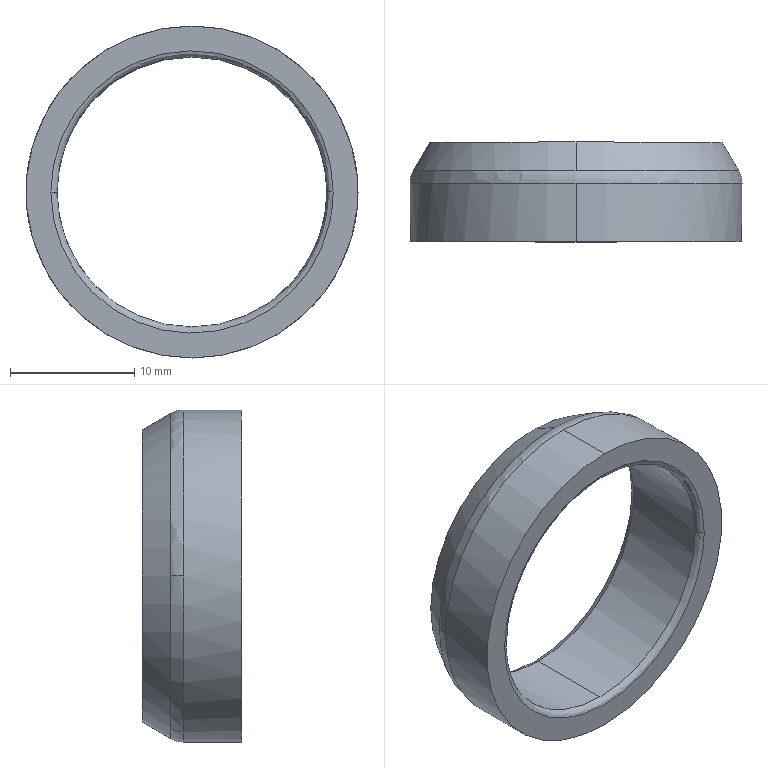Part | STEP file | 00399797_RING_ELASTOMER_MKRT-23-16.5 | 1 solid | 14 faces | box 26.7 x 8 x 26.7 mm | volume 1330 mm3 | spline 4 | cylinder 4 | cone 4 | plane 2 | commonest cylinder face diameters 21.7 x2 26.7 x2